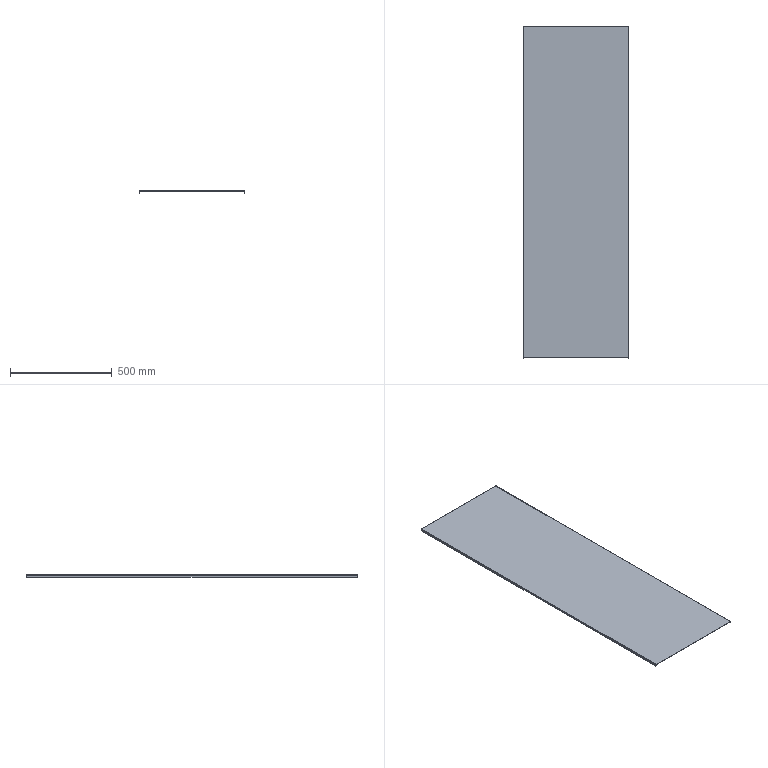Part | STEP file | HESS-408-70-15W-D-12-electrical mounting plate | 1 solid | 18 faces | box 520 x 1630 x 10 mm | volume 1311169 mm3 | plane 10 | cylinder 8 | commonest cylinder face diameters 6 x4 0.2 x2 3.2 x2
STEP:
#1=CARTESIAN_POINT('',(0.,0.,0.));
#2=DIRECTION('',(0.,0.,1.));
#3=DIRECTION('',(1.,0.,0.));
#4=AXIS2_PLACEMENT_3D('',#1,#2,#3);
#5=CARTESIAN_POINT('',(258.4,-815.,-1.5));
#6=VERTEX_POINT('',#5);
#7=CARTESIAN_POINT('',(-258.4,-815.,-1.5));
#8=VERTEX_POINT('',#7);
#9=CARTESIAN_POINT('',(0.,-815.,-1.5));
#10=DIRECTION('',(-1.,0.,0.));
#11=VECTOR('',#10,1.);
#12=LINE('',#9,#11);
#13=CARTESIAN_POINT('',(0.,0.,-1.5));
#14=DIRECTION('',(0.,0.,-1.));
#15=DIRECTION('',(0.,1.,0.));
#16=AXIS2_PLACEMENT_3D('',#13,#14,#15);
#17=PLANE('',#16);
#18=CARTESIAN_POINT('',(-815.,0.));
#19=DIRECTION('',(0.,-1.));
#20=VECTOR('',#19,1.);
#21=LINE('',#18,#20);
#22=(GEOMETRIC_REPRESENTATION_CONTEXT(2)PARAMETRIC_REPRESENTATION_CONTEXT()REPRESENTATION_CONTEXT('',''));
#23=DEFINITIONAL_REPRESENTATION('',(#21),#22);
#24=PCURVE('',#17,#23);
#25=CARTESIAN_POINT('',(-260.,-815.,-1.5));
#26=DIRECTION('',(0.,-1.,0.));
#27=DIRECTION('',(0.,0.,-1.));
#28=AXIS2_PLACEMENT_3D('',#25,#26,#27);
#29=PLANE('',#28);
#30=CARTESIAN_POINT('',(0.,260.));
#31=DIRECTION('',(0.,-1.));
#32=VECTOR('',#31,1.);
#33=LINE('',#30,#32);
#34=(GEOMETRIC_REPRESENTATION_CONTEXT(2)PARAMETRIC_REPRESENTATION_CONTEXT()REPRESENTATION_CONTEXT('',''));
#35=DEFINITIONAL_REPRESENTATION('',(#33),#34);
#36=PCURVE('',#29,#35);
#37=SURFACE_CURVE('',#12,(#24,#36),.PCURVE_S1.);
#38=EDGE_CURVE('',#6,#8,#37,.T.);
#39=ORIENTED_EDGE('',*,*,#38,.T.);
#40=CARTESIAN_POINT('',(-258.4,815.,-1.5));
#41=VERTEX_POINT('',#40);
#42=CARTESIAN_POINT('',(-258.4,0.,-1.5));
#43=DIRECTION('',(0.,1.,0.));
#44=VECTOR('',#43,1.);
#45=LINE('',#42,#44);
#46=CARTESIAN_POINT('',(0.,-258.4));
#47=DIRECTION('',(1.,0.));
#48=VECTOR('',#47,1.);
#49=LINE('',#46,#48);
#50=(GEOMETRIC_REPRESENTATION_CONTEXT(2)PARAMETRIC_REPRESENTATION_CONTEXT()REPRESENTATION_CONTEXT('',''));
#51=DEFINITIONAL_REPRESENTATION('',(#49),#50);
#52=PCURVE('',#17,#51);
#53=CARTESIAN_POINT('',(-258.4,815.,-1.6));
#54=DIRECTION('',(0.,1.,0.));
#55=DIRECTION('',(0.,0.,1.));
#56=AXIS2_PLACEMENT_3D('',#53,#54,#55);
#57=CYLINDRICAL_SURFACE('',#56,0.1);
#58=CARTESIAN_POINT('',(6.283,-815.));
#59=DIRECTION('',(0.,1.));
#60=VECTOR('',#59,1.);
#61=LINE('',#58,#60);
#62=(GEOMETRIC_REPRESENTATION_CONTEXT(2)PARAMETRIC_REPRESENTATION_CONTEXT()REPRESENTATION_CONTEXT('',''));
#63=DEFINITIONAL_REPRESENTATION('',(#61),#62);
#64=PCURVE('',#57,#63);
#65=SURFACE_CURVE('',#45,(#52,#64),.PCURVE_S1.);
#66=EDGE_CURVE('',#8,#41,#65,.T.);
#67=ORIENTED_EDGE('',*,*,#66,.T.);
#68=CARTESIAN_POINT('',(258.4,815.,-1.5));
#69=VERTEX_POINT('',#68);
#70=CARTESIAN_POINT('',(0.,815.,-1.5));
#71=DIRECTION('',(1.,0.,0.));
#72=VECTOR('',#71,1.);
#73=LINE('',#70,#72);
#74=CARTESIAN_POINT('',(815.,0.));
#75=DIRECTION('',(0.,1.));
#76=VECTOR('',#75,1.);
#77=LINE('',#74,#76);
#78=(GEOMETRIC_REPRESENTATION_CONTEXT(2)PARAMETRIC_REPRESENTATION_CONTEXT()REPRESENTATION_CONTEXT('',''));
#79=DEFINITIONAL_REPRESENTATION('',(#77),#78);
#80=PCURVE('',#17,#79);
#81=CARTESIAN_POINT('',(-260.,815.,-1.5));
#82=DIRECTION('',(0.,1.,0.));
#83=DIRECTION('',(0.,0.,1.));
#84=AXIS2_PLACEMENT_3D('',#81,#82,#83);
#85=PLANE('',#84);
#86=CARTESIAN_POINT('',(0.,260.));
#87=DIRECTION('',(0.,1.));
#88=VECTOR('',#87,1.);
#89=LINE('',#86,#88);
#90=(GEOMETRIC_REPRESENTATION_CONTEXT(2)PARAMETRIC_REPRESENTATION_CONTEXT()REPRESENTATION_CONTEXT('',''));
#91=DEFINITIONAL_REPRESENTATION('',(#89),#90);
#92=PCURVE('',#85,#91);
#93=SURFACE_CURVE('',#73,(#80,#92),.PCURVE_S1.);
#94=EDGE_CURVE('',#41,#69,#93,.T.);
#95=ORIENTED_EDGE('',*,*,#94,.T.);
#96=CARTESIAN_POINT('',(258.4,0.,-1.5));
#97=DIRECTION('',(0.,-1.,0.));
#98=VECTOR('',#97,1.);
#99=LINE('',#96,#98);
#100=CARTESIAN_POINT('',(0.,258.4));
#101=DIRECTION('',(-1.,0.));
#102=VECTOR('',#101,1.);
#103=LINE('',#100,#102);
#104=(GEOMETRIC_REPRESENTATION_CONTEXT(2)PARAMETRIC_REPRESENTATION_CONTEXT()REPRESENTATION_CONTEXT('',''));
#105=DEFINITIONAL_REPRESENTATION('',(#103),#104);
#106=PCURVE('',#17,#105);
#107=CARTESIAN_POINT('',(258.4,-815.,-1.6));
#108=DIRECTION('',(0.,-1.,0.));
#109=DIRECTION('',(0.,0.,-1.));
#110=AXIS2_PLACEMENT_3D('',#107,#108,#109);
#111=CYLINDRICAL_SURFACE('',#110,0.1);
#112=CARTESIAN_POINT('',(3.142,-815.));
#113=DIRECTION('',(0.,1.));
#114=VECTOR('',#113,1.);
#115=LINE('',#112,#114);
#116=(GEOMETRIC_REPRESENTATION_CONTEXT(2)PARAMETRIC_REPRESENTATION_CONTEXT()REPRESENTATION_CONTEXT('',''));
#117=DEFINITIONAL_REPRESENTATION('',(#115),#116);
#118=PCURVE('',#111,#117);
#119=SURFACE_CURVE('',#99,(#106,#118),.PCURVE_S1.);
#120=EDGE_CURVE('',#69,#6,#119,.T.);
#121=ORIENTED_EDGE('',*,*,#120,.T.);
#122=EDGE_LOOP('',(#39,#67,#95,#121));
#123=FACE_BOUND('',#122,.T.);
#124=ADVANCED_FACE('',(#123),#17,.T.);
#125=ORIENTED_EDGE('',*,*,#66,.T.);
#126=CARTESIAN_POINT('',(-258.5,815.,-1.6));
#127=VERTEX_POINT('',#126);
#128=CARTESIAN_POINT('',(-258.4,815.,-1.6));
#129=DIRECTION('',(0.,1.,0.));
#130=DIRECTION('',(0.,0.,1.));
#131=AXIS2_PLACEMENT_3D('',#128,#129,#130);
#132=CIRCLE('',#131,0.1);
#133=CARTESIAN_POINT('',(0.,0.));
#134=DIRECTION('',(1.,0.));
#135=VECTOR('',#134,1.);
#136=LINE('',#133,#135);
#137=(GEOMETRIC_REPRESENTATION_CONTEXT(2)PARAMETRIC_REPRESENTATION_CONTEXT()REPRESENTATION_CONTEXT('',''));
#138=DEFINITIONAL_REPRESENTATION('',(#136),#137);
#139=PCURVE('',#57,#138);
#140=CARTESIAN_POINT('',(-0.1,1.6));
#141=DIRECTION('',(1.,0.));
#142=AXIS2_PLACEMENT_2D('',#140,#141);
#143=CIRCLE('',#142,0.1);
#144=(GEOMETRIC_REPRESENTATION_CONTEXT(2)PARAMETRIC_REPRESENTATION_CONTEXT()REPRESENTATION_CONTEXT('',''));
#145=DEFINITIONAL_REPRESENTATION('',(#143),#144);
#146=PCURVE('',#85,#145);
#147=SURFACE_CURVE('',#132,(#139,#146),.PCURVE_S1.);
#148=EDGE_CURVE('',#127,#41,#147,.T.);
#149=ORIENTED_EDGE('',*,*,#148,.F.);
#150=CARTESIAN_POINT('',(-258.5,-815.,-1.6));
#151=VERTEX_POINT('',#150);
#152=CARTESIAN_POINT('',(-258.5,815.,-1.6));
#153=DIRECTION('',(0.,-1.,0.));
#154=VECTOR('',#153,1.);
#155=LINE('',#152,#154);
#156=CARTESIAN_POINT('',(4.712,0.));
#157=DIRECTION('',(0.,-1.));
#158=VECTOR('',#157,1.);
#159=LINE('',#156,#158);
#160=(GEOMETRIC_REPRESENTATION_CONTEXT(2)PARAMETRIC_REPRESENTATION_CONTEXT()REPRESENTATION_CONTEXT('',''));
#161=DEFINITIONAL_REPRESENTATION('',(#159),#160);
#162=PCURVE('',#57,#161);
#163=CARTESIAN_POINT('',(-258.5,0.,0.));
#164=DIRECTION('',(-1.,0.,0.));
#165=DIRECTION('',(0.,0.,1.));
#166=AXIS2_PLACEMENT_3D('',#163,#164,#165);
#167=PLANE('',#166);
#168=CARTESIAN_POINT('',(-1.6,815.));
#169=DIRECTION('',(0.,-1.));
#170=VECTOR('',#169,1.);
#171=LINE('',#168,#170);
#172=(GEOMETRIC_REPRESENTATION_CONTEXT(2)PARAMETRIC_REPRESENTATION_CONTEXT()REPRESENTATION_CONTEXT('',''));
#173=DEFINITIONAL_REPRESENTATION('',(#171),#172);
#174=PCURVE('',#167,#173);
#175=SURFACE_CURVE('',#155,(#162,#174),.PCURVE_S1.);
#176=EDGE_CURVE('',#127,#151,#175,.T.);
#177=ORIENTED_EDGE('',*,*,#176,.T.);
#178=CARTESIAN_POINT('',(-258.4,-815.,-1.6));
#179=DIRECTION('',(0.,1.,0.));
#180=DIRECTION('',(0.,0.,1.));
#181=AXIS2_PLACEMENT_3D('',#178,#179,#180);
#182=CIRCLE('',#181,0.1);
#183=CARTESIAN_POINT('',(0.,-1630.));
#184=DIRECTION('',(1.,0.));
#185=VECTOR('',#184,1.);
#186=LINE('',#183,#185);
#187=(GEOMETRIC_REPRESENTATION_CONTEXT(2)PARAMETRIC_REPRESENTATION_CONTEXT()REPRESENTATION_CONTEXT('',''));
#188=DEFINITIONAL_REPRESENTATION('',(#186),#187);
#189=PCURVE('',#57,#188);
#190=CARTESIAN_POINT('',(0.,1.6));
#191=CARTESIAN_POINT('',(0.,1.773));
#192=CARTESIAN_POINT('',(0.15,1.687));
#193=CARTESIAN_POINT('',(0.3,1.6));
#194=CARTESIAN_POINT('',(0.15,1.513));
#195=CARTESIAN_POINT('',(0.,1.427));
#196=CARTESIAN_POINT('',(0.,1.6));
#197=(BOUNDED_CURVE()B_SPLINE_CURVE(2,(#190,#191,#192,#193,#194,#195,#196),.UNSPECIFIED.,.T.,.F.)B_SPLINE_CURVE_WITH_KNOTS((1,2,2,2,2,1),(-2.094,0.,2.094,4.189,6.283,8.378),.UNSPECIFIED.)CURVE()GEOMETRIC_REPRESENTATION_ITEM()RATIONAL_B_SPLINE_CURVE((1.,0.5,1.,0.5,1.,0.5,1.))REPRESENTATION_ITEM(''));
#198=(GEOMETRIC_REPRESENTATION_CONTEXT(2)PARAMETRIC_REPRESENTATION_CONTEXT()REPRESENTATION_CONTEXT('',''));
#199=DEFINITIONAL_REPRESENTATION('',(#197),#198);
#200=PCURVE('',#29,#199);
#201=SURFACE_CURVE('',#182,(#189,#200),.PCURVE_S1.);
#202=EDGE_CURVE('',#151,#8,#201,.T.);
#203=ORIENTED_EDGE('',*,*,#202,.T.);
#204=EDGE_LOOP('',(#125,#149,#177,#203));
#205=FACE_BOUND('',#204,.F.);
#206=ADVANCED_FACE('',(#205),#57,.F.);
#207=CARTESIAN_POINT('',(258.4,-815.,0.));
#208=VERTEX_POINT('',#207);
#209=CARTESIAN_POINT('',(-258.4,-815.,0.));
#210=VERTEX_POINT('',#209);
#211=CARTESIAN_POINT('',(-260.,-815.,0.));
#212=DIRECTION('',(-1.,0.,0.));
#213=VECTOR('',#212,1.);
#214=LINE('',#211,#213);
#215=CARTESIAN_POINT('',(-1.5,0.));
#216=DIRECTION('',(0.,-1.));
#217=VECTOR('',#216,1.);
#218=LINE('',#215,#217);
#219=(GEOMETRIC_REPRESENTATION_CONTEXT(2)PARAMETRIC_REPRESENTATION_CONTEXT()REPRESENTATION_CONTEXT('',''));
#220=DEFINITIONAL_REPRESENTATION('',(#218),#219);
#221=PCURVE('',#29,#220);
#222=CARTESIAN_POINT('',(0.,0.,0.));
#223=DIRECTION('',(0.,0.,-1.));
#224=DIRECTION('',(0.,1.,0.));
#225=AXIS2_PLACEMENT_3D('',#222,#223,#224);
#226=PLANE('',#225);
#227=CARTESIAN_POINT('',(-815.,-260.));
#228=DIRECTION('',(0.,-1.));
#229=VECTOR('',#228,1.);
#230=LINE('',#227,#229);
#231=(GEOMETRIC_REPRESENTATION_CONTEXT(2)PARAMETRIC_REPRESENTATION_CONTEXT()REPRESENTATION_CONTEXT('',''));
#232=DEFINITIONAL_REPRESENTATION('',(#230),#231);
#233=PCURVE('',#226,#232);
#234=SURFACE_CURVE('',#214,(#221,#233),.PCURVE_S1.);
#235=EDGE_CURVE('',#208,#210,#234,.T.);
#236=ORIENTED_EDGE('',*,*,#235,.T.);
#237=CARTESIAN_POINT('',(-260.,-815.,-1.6));
#238=VERTEX_POINT('',#237);
#239=CARTESIAN_POINT('',(-258.4,-815.,-1.6));
#240=DIRECTION('',(0.,1.,0.));
#241=DIRECTION('',(0.,0.,1.));
#242=AXIS2_PLACEMENT_3D('',#239,#240,#241);
#243=CIRCLE('',#242,1.6);
#244=CARTESIAN_POINT('',(-1.5,1.6));
#245=CARTESIAN_POINT('',(-1.5,4.371));
#246=CARTESIAN_POINT('',(0.9,2.986));
#247=CARTESIAN_POINT('',(3.3,1.6));
#248=CARTESIAN_POINT('',(0.9,0.2144));
#249=CARTESIAN_POINT('',(-1.5,-1.171));
#250=CARTESIAN_POINT('',(-1.5,1.6));
#251=(BOUNDED_CURVE()B_SPLINE_CURVE(2,(#244,#245,#246,#247,#248,#249,#250),.UNSPECIFIED.,.T.,.F.)B_SPLINE_CURVE_WITH_KNOTS((1,2,2,2,2,1),(-2.094,0.,2.094,4.189,6.283,8.378),.UNSPECIFIED.)CURVE()GEOMETRIC_REPRESENTATION_ITEM()RATIONAL_B_SPLINE_CURVE((1.,0.5,1.,0.5,1.,0.5,1.))REPRESENTATION_ITEM(''));
#252=(GEOMETRIC_REPRESENTATION_CONTEXT(2)PARAMETRIC_REPRESENTATION_CONTEXT()REPRESENTATION_CONTEXT('',''));
#253=DEFINITIONAL_REPRESENTATION('',(#251),#252);
#254=PCURVE('',#29,#253);
#255=CARTESIAN_POINT('',(-258.4,815.,-1.6));
#256=DIRECTION('',(0.,1.,0.));
#257=DIRECTION('',(0.,0.,1.));
#258=AXIS2_PLACEMENT_3D('',#255,#256,#257);
#259=CYLINDRICAL_SURFACE('',#258,1.6);
#260=CARTESIAN_POINT('',(0.,-1630.));
#261=DIRECTION('',(1.,0.));
#262=VECTOR('',#261,1.);
#263=LINE('',#260,#262);
#264=(GEOMETRIC_REPRESENTATION_CONTEXT(2)PARAMETRIC_REPRESENTATION_CONTEXT()REPRESENTATION_CONTEXT('',''));
#265=DEFINITIONAL_REPRESENTATION('',(#263),#264);
#266=PCURVE('',#259,#265);
#267=SURFACE_CURVE('',#243,(#254,#266),.PCURVE_S1.);
#268=EDGE_CURVE('',#238,#210,#267,.T.);
#269=ORIENTED_EDGE('',*,*,#268,.F.);
#270=CARTESIAN_POINT('',(-260.,-815.,-7.));
#271=VERTEX_POINT('',#270);
#272=CARTESIAN_POINT('',(-260.,-815.,-10.));
#273=DIRECTION('',(0.,0.,-1.));
#274=VECTOR('',#273,1.);
#275=LINE('',#272,#274);
#276=CARTESIAN_POINT('',(8.5,0.));
#277=DIRECTION('',(1.,0.));
#278=VECTOR('',#277,1.);
#279=LINE('',#276,#278);
#280=(GEOMETRIC_REPRESENTATION_CONTEXT(2)PARAMETRIC_REPRESENTATION_CONTEXT()REPRESENTATION_CONTEXT('',''));
#281=DEFINITIONAL_REPRESENTATION('',(#279),#280);
#282=PCURVE('',#29,#281);
#283=CARTESIAN_POINT('',(-260.,0.,0.));
#284=DIRECTION('',(-1.,0.,0.));
#285=DIRECTION('',(0.,0.,1.));
#286=AXIS2_PLACEMENT_3D('',#283,#284,#285);
#287=PLANE('',#286);
#288=CARTESIAN_POINT('',(-10.,-815.));
#289=DIRECTION('',(-1.,0.));
#290=VECTOR('',#289,1.);
#291=LINE('',#288,#290);
#292=(GEOMETRIC_REPRESENTATION_CONTEXT(2)PARAMETRIC_REPRESENTATION_CONTEXT()REPRESENTATION_CONTEXT('',''));
#293=DEFINITIONAL_REPRESENTATION('',(#291),#292);
#294=PCURVE('',#287,#293);
#295=SURFACE_CURVE('',#275,(#282,#294),.PCURVE_S1.);
#296=EDGE_CURVE('',#238,#271,#295,.T.);
#297=ORIENTED_EDGE('',*,*,#296,.T.);
#298=CARTESIAN_POINT('',(-258.5,-815.,-7.));
#299=VERTEX_POINT('',#298);
#300=CARTESIAN_POINT('',(-260.,-815.,-7.));
#301=DIRECTION('',(1.,0.,0.));
#302=VECTOR('',#301,1.);
#303=LINE('',#300,#302);
#304=CARTESIAN_POINT('',(5.5,0.));
#305=DIRECTION('',(0.,1.));
#306=VECTOR('',#305,1.);
#307=LINE('',#304,#306);
#308=(GEOMETRIC_REPRESENTATION_CONTEXT(2)PARAMETRIC_REPRESENTATION_CONTEXT()REPRESENTATION_CONTEXT('',''));
#309=DEFINITIONAL_REPRESENTATION('',(#307),#308);
#310=PCURVE('',#29,#309);
#311=CARTESIAN_POINT('',(-260.,-812.,-7.));
#312=DIRECTION('',(1.,0.,0.));
#313=DIRECTION('',(0.,0.,-1.));
#314=AXIS2_PLACEMENT_3D('',#311,#312,#313);
#315=CYLINDRICAL_SURFACE('',#314,3.);
#316=CARTESIAN_POINT('',(4.712,0.));
#317=DIRECTION('',(0.,1.));
#318=VECTOR('',#317,1.);
#319=LINE('',#316,#318);
#320=(GEOMETRIC_REPRESENTATION_CONTEXT(2)PARAMETRIC_REPRESENTATION_CONTEXT()REPRESENTATION_CONTEXT('',''));
#321=DEFINITIONAL_REPRESENTATION('',(#319),#320);
#322=PCURVE('',#315,#321);
#323=SURFACE_CURVE('',#303,(#310,#322),.PCURVE_S1.);
#324=EDGE_CURVE('',#271,#299,#323,.T.);
#325=ORIENTED_EDGE('',*,*,#324,.T.);
#326=CARTESIAN_POINT('',(-258.5,-815.,0.));
#327=DIRECTION('',(0.,0.,1.));
#328=VECTOR('',#327,1.);
#329=LINE('',#326,#328);
#330=CARTESIAN_POINT('',(-1.5,1.5));
#331=DIRECTION('',(-1.,0.));
#332=VECTOR('',#331,1.);
#333=LINE('',#330,#332);
#334=(GEOMETRIC_REPRESENTATION_CONTEXT(2)PARAMETRIC_REPRESENTATION_CONTEXT()REPRESENTATION_CONTEXT('',''));
#335=DEFINITIONAL_REPRESENTATION('',(#333),#334);
#336=PCURVE('',#29,#335);
#337=CARTESIAN_POINT('',(0.,-815.));
#338=DIRECTION('',(1.,0.));
#339=VECTOR('',#338,1.);
#340=LINE('',#337,#339);
#341=(GEOMETRIC_REPRESENTATION_CONTEXT(2)PARAMETRIC_REPRESENTATION_CONTEXT()REPRESENTATION_CONTEXT('',''));
#342=DEFINITIONAL_REPRESENTATION('',(#340),#341);
#343=PCURVE('',#167,#342);
#344=SURFACE_CURVE('',#329,(#336,#343),.PCURVE_S1.);
#345=EDGE_CURVE('',#299,#151,#344,.T.);
#346=ORIENTED_EDGE('',*,*,#345,.T.);
#347=ORIENTED_EDGE('',*,*,#202,.T.);
#348=ORIENTED_EDGE('',*,*,#38,.F.);
#349=CARTESIAN_POINT('',(258.5,-815.,-1.6));
#350=VERTEX_POINT('',#349);
#351=CARTESIAN_POINT('',(258.4,-815.,-1.6));
#352=DIRECTION('',(0.,-1.,0.));
#353=DIRECTION('',(0.,0.,-1.));
#354=AXIS2_PLACEMENT_3D('',#351,#352,#353);
#355=CIRCLE('',#354,0.1);
#356=CARTESIAN_POINT('',(0.1,518.4));
#357=DIRECTION('',(1.,0.));
#358=AXIS2_PLACEMENT_2D('',#356,#357);
#359=CIRCLE('',#358,0.1);
#360=(GEOMETRIC_REPRESENTATION_CONTEXT(2)PARAMETRIC_REPRESENTATION_CONTEXT()REPRESENTATION_CONTEXT('',''));
#361=DEFINITIONAL_REPRESENTATION('',(#359),#360);
#362=PCURVE('',#29,#361);
#363=CARTESIAN_POINT('',(0.,0.));
#364=DIRECTION('',(1.,0.));
#365=VECTOR('',#364,1.);
#366=LINE('',#363,#365);
#367=(GEOMETRIC_REPRESENTATION_CONTEXT(2)PARAMETRIC_REPRESENTATION_CONTEXT()REPRESENTATION_CONTEXT('',''));
#368=DEFINITIONAL_REPRESENTATION('',(#366),#367);
#369=PCURVE('',#111,#368);
#370=SURFACE_CURVE('',#355,(#362,#369),.PCURVE_S1.);
#371=EDGE_CURVE('',#350,#6,#370,.T.);
#372=ORIENTED_EDGE('',*,*,#371,.F.);
#373=CARTESIAN_POINT('',(258.5,-815.,-7.));
#374=VERTEX_POINT('',#373);
#375=CARTESIAN_POINT('',(258.5,-815.,0.));
#376=DIRECTION('',(0.,0.,1.));
#377=VECTOR('',#376,1.);
#378=LINE('',#375,#377);
#379=CARTESIAN_POINT('',(-1.5,518.5));
#380=DIRECTION('',(-1.,0.));
#381=VECTOR('',#380,1.);
#382=LINE('',#379,#381);
#383=(GEOMETRIC_REPRESENTATION_CONTEXT(2)PARAMETRIC_REPRESENTATION_CONTEXT()REPRESENTATION_CONTEXT('',''));
#384=DEFINITIONAL_REPRESENTATION('',(#382),#383);
#385=PCURVE('',#29,#384);
#386=CARTESIAN_POINT('',(258.5,0.,0.));
#387=DIRECTION('',(-1.,0.,0.));
#388=DIRECTION('',(0.,0.,1.));
#389=AXIS2_PLACEMENT_3D('',#386,#387,#388);
#390=PLANE('',#389);
#391=CARTESIAN_POINT('',(0.,-815.));
#392=DIRECTION('',(1.,0.));
#393=VECTOR('',#392,1.);
#394=LINE('',#391,#393);
#395=(GEOMETRIC_REPRESENTATION_CONTEXT(2)PARAMETRIC_REPRESENTATION_CONTEXT()REPRESENTATION_CONTEXT('',''));
#396=DEFINITIONAL_REPRESENTATION('',(#394),#395);
#397=PCURVE('',#390,#396);
#398=SURFACE_CURVE('',#378,(#385,#397),.PCURVE_S1.);
#399=EDGE_CURVE('',#374,#350,#398,.T.);
#400=ORIENTED_EDGE('',*,*,#399,.F.);
#401=CARTESIAN_POINT('',(260.,-815.,-7.));
#402=VERTEX_POINT('',#401);
#403=CARTESIAN_POINT('',(260.,-815.,-7.));
#404=DIRECTION('',(1.,0.,0.));
#405=VECTOR('',#404,1.);
#406=LINE('',#403,#405);
#407=CARTESIAN_POINT('',(5.5,520.));
#408=DIRECTION('',(0.,1.));
#409=VECTOR('',#408,1.);
#410=LINE('',#407,#409);
#411=(GEOMETRIC_REPRESENTATION_CONTEXT(2)PARAMETRIC_REPRESENTATION_CONTEXT()REPRESENTATION_CONTEXT('',''));
#412=DEFINITIONAL_REPRESENTATION('',(#410),#411);
#413=PCURVE('',#29,#412);
#414=CARTESIAN_POINT('',(260.,-812.,-7.));
#415=DIRECTION('',(-1.,0.,0.));
#416=DIRECTION('',(0.,0.,1.));
#417=AXIS2_PLACEMENT_3D('',#414,#415,#416);
#418=CYLINDRICAL_SURFACE('',#417,3.);
#419=CARTESIAN_POINT('',(4.712,0.));
#420=DIRECTION('',(0.,-1.));
#421=VECTOR('',#420,1.);
#422=LINE('',#419,#421);
#423=(GEOMETRIC_REPRESENTATION_CONTEXT(2)PARAMETRIC_REPRESENTATION_CONTEXT()REPRESENTATION_CONTEXT('',''));
#424=DEFINITIONAL_REPRESENTATION('',(#422),#423);
#425=PCURVE('',#418,#424);
#426=SURFACE_CURVE('',#406,(#413,#425),.PCURVE_S1.);
#427=EDGE_CURVE('',#374,#402,#426,.T.);
#428=ORIENTED_EDGE('',*,*,#427,.T.);
#429=CARTESIAN_POINT('',(260.,-815.,-1.6));
#430=VERTEX_POINT('',#429);
#431=CARTESIAN_POINT('',(260.,-815.,-10.));
#432=DIRECTION('',(0.,0.,1.));
#433=VECTOR('',#432,1.);
#434=LINE('',#431,#433);
#435=CARTESIAN_POINT('',(8.5,520.));
#436=DIRECTION('',(-1.,0.));
#437=VECTOR('',#436,1.);
#438=LINE('',#435,#437);
#439=(GEOMETRIC_REPRESENTATION_CONTEXT(2)PARAMETRIC_REPRESENTATION_CONTEXT()REPRESENTATION_CONTEXT('',''));
#440=DEFINITIONAL_REPRESENTATION('',(#438),#439);
#441=PCURVE('',#29,#440);
#442=CARTESIAN_POINT('',(260.,0.,0.));
#443=DIRECTION('',(-1.,0.,0.));
#444=DIRECTION('',(0.,0.,1.));
#445=AXIS2_PLACEMENT_3D('',#442,#443,#444);
#446=PLANE('',#445);
#447=CARTESIAN_POINT('',(-10.,-815.));
#448=DIRECTION('',(1.,0.));
#449=VECTOR('',#448,1.);
#450=LINE('',#447,#449);
#451=(GEOMETRIC_REPRESENTATION_CONTEXT(2)PARAMETRIC_REPRESENTATION_CONTEXT()REPRESENTATION_CONTEXT('',''));
#452=DEFINITIONAL_REPRESENTATION('',(#450),#451);
#453=PCURVE('',#446,#452);
#454=SURFACE_CURVE('',#434,(#441,#453),.PCURVE_S1.);
#455=EDGE_CURVE('',#402,#430,#454,.T.);
#456=ORIENTED_EDGE('',*,*,#455,.T.);
#457=CARTESIAN_POINT('',(258.4,-815.,-1.6));
#458=DIRECTION('',(0.,1.,0.));
#459=DIRECTION('',(0.,0.,-1.));
#460=AXIS2_PLACEMENT_3D('',#457,#458,#459);
#461=CIRCLE('',#460,1.6);
#462=CARTESIAN_POINT('',(1.7,518.4));
#463=CARTESIAN_POINT('',(1.7,515.629));
#464=CARTESIAN_POINT('',(-0.7,517.014));
#465=CARTESIAN_POINT('',(-3.1,518.4));
#466=CARTESIAN_POINT('',(-0.7,519.786));
#467=CARTESIAN_POINT('',(1.7,521.171));
#468=CARTESIAN_POINT('',(1.7,518.4));
#469=(BOUNDED_CURVE()B_SPLINE_CURVE(2,(#462,#463,#464,#465,#466,#467,#468),.UNSPECIFIED.,.T.,.F.)B_SPLINE_CURVE_WITH_KNOTS((1,2,2,2,2,1),(-2.094,0.,2.094,4.189,6.283,8.378),.UNSPECIFIED.)CURVE()GEOMETRIC_REPRESENTATION_ITEM()RATIONAL_B_SPLINE_CURVE((1.,0.5,1.,0.5,1.,0.5,1.))REPRESENTATION_ITEM(''));
#470=(GEOMETRIC_REPRESENTATION_CONTEXT(2)PARAMETRIC_REPRESENTATION_CONTEXT()REPRESENTATION_CONTEXT('',''));
#471=DEFINITIONAL_REPRESENTATION('',(#469),#470);
#472=PCURVE('',#29,#471);
#473=CARTESIAN_POINT('',(258.4,-815.,-1.6));
#474=DIRECTION('',(0.,-1.,0.));
#475=DIRECTION('',(0.,0.,-1.));
#476=AXIS2_PLACEMENT_3D('',#473,#474,#475);
#477=CYLINDRICAL_SURFACE('',#476,1.6);
#478=CARTESIAN_POINT('',(6.283,0.));
#479=DIRECTION('',(-1.,0.));
#480=VECTOR('',#479,1.);
#481=LINE('',#478,#480);
#482=(GEOMETRIC_REPRESENTATION_CONTEXT(2)PARAMETRIC_REPRESENTATION_CONTEXT()REPRESENTATION_CONTEXT('',''));
#483=DEFINITIONAL_REPRESENTATION('',(#481),#482);
#484=PCURVE('',#477,#483);
#485=SURFACE_CURVE('',#461,(#472,#484),.PCURVE_S1.);
#486=EDGE_CURVE('',#208,#430,#485,.T.);
#487=ORIENTED_EDGE('',*,*,#486,.F.);
#488=EDGE_LOOP('',(#236,#269,#297,#325,#346,#347,#348,#372,#400,#428,#456,#487));
#489=FACE_BOUND('',#488,.T.);
#490=ADVANCED_FACE('',(#489),#29,.T.);
#491=ORIENTED_EDGE('',*,*,#120,.T.);
#492=ORIENTED_EDGE('',*,*,#371,.F.);
#493=CARTESIAN_POINT('',(258.5,815.,-1.6));
#494=VERTEX_POINT('',#493);
#495=CARTESIAN_POINT('',(258.5,-815.,-1.6));
#496=DIRECTION('',(0.,1.,0.));
#497=VECTOR('',#496,1.);
#498=LINE('',#495,#497);
#499=CARTESIAN_POINT('',(1.571,0.));
#500=DIRECTION('',(0.,-1.));
#501=VECTOR('',#500,1.);
#502=LINE('',#499,#501);
#503=(GEOMETRIC_REPRESENTATION_CONTEXT(2)PARAMETRIC_REPRESENTATION_CONTEXT()REPRESENTATION_CONTEXT('',''));
#504=DEFINITIONAL_REPRESENTATION('',(#502),#503);
#505=PCURVE('',#111,#504);
#506=CARTESIAN_POINT('',(-1.6,-815.));
#507=DIRECTION('',(0.,1.));
#508=VECTOR('',#507,1.);
#509=LINE('',#506,#508);
#510=(GEOMETRIC_REPRESENTATION_CONTEXT(2)PARAMETRIC_REPRESENTATION_CONTEXT()REPRESENTATION_CONTEXT('',''));
#511=DEFINITIONAL_REPRESENTATION('',(#509),#510);
#512=PCURVE('',#390,#511);
#513=SURFACE_CURVE('',#498,(#505,#512),.PCURVE_S1.);
#514=EDGE_CURVE('',#350,#494,#513,.T.);
#515=ORIENTED_EDGE('',*,*,#514,.T.);
#516=CARTESIAN_POINT('',(258.4,815.,-1.6));
#517=DIRECTION('',(0.,-1.,0.));
#518=DIRECTION('',(0.,0.,-1.));
#519=AXIS2_PLACEMENT_3D('',#516,#517,#518);
#520=CIRCLE('',#519,0.1);
#521=CARTESIAN_POINT('',(0.,-1630.));
#522=DIRECTION('',(1.,0.));
#523=VECTOR('',#522,1.);
#524=LINE('',#521,#523);
#525=(GEOMETRIC_REPRESENTATION_CONTEXT(2)PARAMETRIC_REPRESENTATION_CONTEXT()REPRESENTATION_CONTEXT('',''));
#526=DEFINITIONAL_REPRESENTATION('',(#524),#525);
#527=PCURVE('',#111,#526);
#528=CARTESIAN_POINT('',(-0.2,518.4));
#529=CARTESIAN_POINT('',(-0.2,518.573));
#530=CARTESIAN_POINT('',(-0.05,518.487));
#531=CARTESIAN_POINT('',(0.1,518.4));
#532=CARTESIAN_POINT('',(-0.05,518.313));
#533=CARTESIAN_POINT('',(-0.2,518.227));
#534=CARTESIAN_POINT('',(-0.2,518.4));
#535=(BOUNDED_CURVE()B_SPLINE_CURVE(2,(#528,#529,#530,#531,#532,#533,#534),.UNSPECIFIED.,.T.,.F.)B_SPLINE_CURVE_WITH_KNOTS((1,2,2,2,2,1),(-2.094,0.,2.094,4.189,6.283,8.378),.UNSPECIFIED.)CURVE()GEOMETRIC_REPRESENTATION_ITEM()RATIONAL_B_SPLINE_CURVE((1.,0.5,1.,0.5,1.,0.5,1.))REPRESENTATION_ITEM(''));
#536=(GEOMETRIC_REPRESENTATION_CONTEXT(2)PARAMETRIC_REPRESENTATION_CONTEXT()REPRESENTATION_CONTEXT('',''));
#537=DEFINITIONAL_REPRESENTATION('',(#535),#536);
#538=PCURVE('',#85,#537);
#539=SURFACE_CURVE('',#520,(#527,#538),.PCURVE_S1.);
#540=EDGE_CURVE('',#494,#69,#539,.T.);
#541=ORIENTED_EDGE('',*,*,#540,.T.);
#542=EDGE_LOOP('',(#491,#492,#515,#541));
#543=FACE_BOUND('',#542,.F.);
#544=ADVANCED_FACE('',(#543),#111,.F.);
#545=ORIENTED_EDGE('',*,*,#94,.F.);
#546=ORIENTED_EDGE('',*,*,#148,.F.);
#547=CARTESIAN_POINT('',(-258.5,815.,-7.));
#548=VERTEX_POINT('',#547);
#549=CARTESIAN_POINT('',(-258.5,815.,0.));
#550=DIRECTION('',(0.,0.,-1.));
#551=VECTOR('',#550,1.);
#552=LINE('',#549,#551);
#553=CARTESIAN_POINT('',(1.5,1.5));
#554=DIRECTION('',(-1.,0.));
#555=VECTOR('',#554,1.);
#556=LINE('',#553,#555);
#557=(GEOMETRIC_REPRESENTATION_CONTEXT(2)PARAMETRIC_REPRESENTATION_CONTEXT()REPRESENTATION_CONTEXT('',''));
#558=DEFINITIONAL_REPRESENTATION('',(#556),#557);
#559=PCURVE('',#85,#558);
#560=CARTESIAN_POINT('',(0.,815.));
#561=DIRECTION('',(-1.,0.));
#562=VECTOR('',#561,1.);
#563=LINE('',#560,#562);
#564=(GEOMETRIC_REPRESENTATION_CONTEXT(2)PARAMETRIC_REPRESENTATION_CONTEXT()REPRESENTATION_CONTEXT('',''));
#565=DEFINITIONAL_REPRESENTATION('',(#563),#564);
#566=PCURVE('',#167,#565);
#567=SURFACE_CURVE('',#552,(#559,#566),.PCURVE_S1.);
#568=EDGE_CURVE('',#127,#548,#567,.T.);
#569=ORIENTED_EDGE('',*,*,#568,.T.);
#570=CARTESIAN_POINT('',(-260.,815.,-7.));
#571=VERTEX_POINT('',#570);
#572=CARTESIAN_POINT('',(-260.,815.,-7.));
#573=DIRECTION('',(1.,0.,0.));
#574=VECTOR('',#573,1.);
#575=LINE('',#572,#574);
#576=CARTESIAN_POINT('',(-5.5,0.));
#577=DIRECTION('',(0.,1.));
#578=VECTOR('',#577,1.);
#579=LINE('',#576,#578);
#580=(GEOMETRIC_REPRESENTATION_CONTEXT(2)PARAMETRIC_REPRESENTATION_CONTEXT()REPRESENTATION_CONTEXT('',''));
#581=DEFINITIONAL_REPRESENTATION('',(#579),#580);
#582=PCURVE('',#85,#581);
#583=CARTESIAN_POINT('',(-260.,812.,-7.));
#584=DIRECTION('',(1.,0.,0.));
#585=DIRECTION('',(0.,0.,-1.));
#586=AXIS2_PLACEMENT_3D('',#583,#584,#585);
#587=CYLINDRICAL_SURFACE('',#586,3.);
#588=CARTESIAN_POINT('',(1.571,0.));
#589=DIRECTION('',(0.,1.));
#590=VECTOR('',#589,1.);
#591=LINE('',#588,#590);
#592=(GEOMETRIC_REPRESENTATION_CONTEXT(2)PARAMETRIC_REPRESENTATION_CONTEXT()REPRESENTATION_CONTEXT('',''));
#593=DEFINITIONAL_REPRESENTATION('',(#591),#592);
#594=PCURVE('',#587,#593);
#595=SURFACE_CURVE('',#575,(#582,#594),.PCURVE_S1.);
#596=EDGE_CURVE('',#571,#548,#595,.T.);
#597=ORIENTED_EDGE('',*,*,#596,.F.);
#598=CARTESIAN_POINT('',(-260.,815.,-1.6));
#599=VERTEX_POINT('',#598);
#600=CARTESIAN_POINT('',(-260.,815.,-1.5));
#601=DIRECTION('',(0.,0.,1.));
#602=VECTOR('',#601,1.);
#603=LINE('',#600,#602);
#604=CARTESIAN_POINT('',(0.,0.));
#605=DIRECTION('',(1.,0.));
#606=VECTOR('',#605,1.);
#607=LINE('',#604,#606);
#608=(GEOMETRIC_REPRESENTATION_CONTEXT(2)PARAMETRIC_REPRESENTATION_CONTEXT()REPRESENTATION_CONTEXT('',''));
#609=DEFINITIONAL_REPRESENTATION('',(#607),#608);
#610=PCURVE('',#85,#609);
#611=CARTESIAN_POINT('',(-1.5,815.));
#612=DIRECTION('',(1.,0.));
#613=VECTOR('',#612,1.);
#614=LINE('',#611,#613);
#615=(GEOMETRIC_REPRESENTATION_CONTEXT(2)PARAMETRIC_REPRESENTATION_CONTEXT()REPRESENTATION_CONTEXT('',''));
#616=DEFINITIONAL_REPRESENTATION('',(#614),#615);
#617=PCURVE('',#287,#616);
#618=SURFACE_CURVE('',#603,(#610,#617),.PCURVE_S1.);
#619=EDGE_CURVE('',#571,#599,#618,.T.);
#620=ORIENTED_EDGE('',*,*,#619,.T.);
#621=CARTESIAN_POINT('',(-258.4,815.,0.));
#622=VERTEX_POINT('',#621);
#623=CARTESIAN_POINT('',(-258.4,815.,-1.6));
#624=DIRECTION('',(0.,-1.,0.));
#625=DIRECTION('',(0.,0.,1.));
#626=AXIS2_PLACEMENT_3D('',#623,#624,#625);
#627=CIRCLE('',#626,1.6);
#628=CARTESIAN_POINT('',(1.5,1.6));
#629=CARTESIAN_POINT('',(1.5,-1.171));
#630=CARTESIAN_POINT('',(-0.9,0.2144));
#631=CARTESIAN_POINT('',(-3.3,1.6));
#632=CARTESIAN_POINT('',(-0.9,2.986));
#633=CARTESIAN_POINT('',(1.5,4.371));
#634=CARTESIAN_POINT('',(1.5,1.6));
#635=(BOUNDED_CURVE()B_SPLINE_CURVE(2,(#628,#629,#630,#631,#632,#633,#634),.UNSPECIFIED.,.T.,.F.)B_SPLINE_CURVE_WITH_KNOTS((1,2,2,2,2,1),(-2.094,0.,2.094,4.189,6.283,8.378),.UNSPECIFIED.)CURVE()GEOMETRIC_REPRESENTATION_ITEM()RATIONAL_B_SPLINE_CURVE((1.,0.5,1.,0.5,1.,0.5,1.))REPRESENTATION_ITEM(''));
#636=(GEOMETRIC_REPRESENTATION_CONTEXT(2)PARAMETRIC_REPRESENTATION_CONTEXT()REPRESENTATION_CONTEXT('',''));
#637=DEFINITIONAL_REPRESENTATION('',(#635),#636);
#638=PCURVE('',#85,#637);
#639=CARTESIAN_POINT('',(6.283,0.));
#640=DIRECTION('',(-1.,0.));
#641=VECTOR('',#640,1.);
#642=LINE('',#639,#641);
#643=(GEOMETRIC_REPRESENTATION_CONTEXT(2)PARAMETRIC_REPRESENTATION_CONTEXT()REPRESENTATION_CONTEXT('',''));
#644=DEFINITIONAL_REPRESENTATION('',(#642),#643);
#645=PCURVE('',#259,#644);
#646=SURFACE_CURVE('',#627,(#638,#645),.PCURVE_S1.);
#647=EDGE_CURVE('',#622,#599,#646,.T.);
#648=ORIENTED_EDGE('',*,*,#647,.F.);
#649=CARTESIAN_POINT('',(258.4,815.,0.));
#650=VERTEX_POINT('',#649);
#651=CARTESIAN_POINT('',(-260.,815.,0.));
#652=DIRECTION('',(1.,0.,0.));
#653=VECTOR('',#652,1.);
#654=LINE('',#651,#653);
#655=CARTESIAN_POINT('',(1.5,0.));
#656=DIRECTION('',(0.,1.));
#657=VECTOR('',#656,1.);
#658=LINE('',#655,#657);
#659=(GEOMETRIC_REPRESENTATION_CONTEXT(2)PARAMETRIC_REPRESENTATION_CONTEXT()REPRESENTATION_CONTEXT('',''));
#660=DEFINITIONAL_REPRESENTATION('',(#658),#659);
#661=PCURVE('',#85,#660);
#662=CARTESIAN_POINT('',(815.,-260.));
#663=DIRECTION('',(0.,1.));
#664=VECTOR('',#663,1.);
#665=LINE('',#662,#664);
#666=(GEOMETRIC_REPRESENTATION_CONTEXT(2)PARAMETRIC_REPRESENTATION_CONTEXT()REPRESENTATION_CONTEXT('',''));
#667=DEFINITIONAL_REPRESENTATION('',(#665),#666);
#668=PCURVE('',#226,#667);
#669=SURFACE_CURVE('',#654,(#661,#668),.PCURVE_S1.);
#670=EDGE_CURVE('',#622,#650,#669,.T.);
#671=ORIENTED_EDGE('',*,*,#670,.T.);
#672=CARTESIAN_POINT('',(260.,815.,-1.6));
#673=VERTEX_POINT('',#672);
#674=CARTESIAN_POINT('',(258.4,815.,-1.6));
#675=DIRECTION('',(0.,-1.,0.));
#676=DIRECTION('',(0.,0.,-1.));
#677=AXIS2_PLACEMENT_3D('',#674,#675,#676);
#678=CIRCLE('',#677,1.6);
#679=CARTESIAN_POINT('',(-1.7,518.4));
#680=CARTESIAN_POINT('',(-1.7,521.171));
#681=CARTESIAN_POINT('',(0.7,519.786));
#682=CARTESIAN_POINT('',(3.1,518.4));
#683=CARTESIAN_POINT('',(0.7,517.014));
#684=CARTESIAN_POINT('',(-1.7,515.629));
#685=CARTESIAN_POINT('',(-1.7,518.4));
#686=(BOUNDED_CURVE()B_SPLINE_CURVE(2,(#679,#680,#681,#682,#683,#684,#685),.UNSPECIFIED.,.T.,.F.)B_SPLINE_CURVE_WITH_KNOTS((1,2,2,2,2,1),(-2.094,0.,2.094,4.189,6.283,8.378),.UNSPECIFIED.)CURVE()GEOMETRIC_REPRESENTATION_ITEM()RATIONAL_B_SPLINE_CURVE((1.,0.5,1.,0.5,1.,0.5,1.))REPRESENTATION_ITEM(''));
#687=(GEOMETRIC_REPRESENTATION_CONTEXT(2)PARAMETRIC_REPRESENTATION_CONTEXT()REPRESENTATION_CONTEXT('',''));
#688=DEFINITIONAL_REPRESENTATION('',(#686),#687);
#689=PCURVE('',#85,#688);
#690=CARTESIAN_POINT('',(0.,-1630.));
#691=DIRECTION('',(1.,0.));
#692=VECTOR('',#691,1.);
#693=LINE('',#690,#692);
#694=(GEOMETRIC_REPRESENTATION_CONTEXT(2)PARAMETRIC_REPRESENTATION_CONTEXT()REPRESENTATION_CONTEXT('',''));
#695=DEFINITIONAL_REPRESENTATION('',(#693),#694);
#696=PCURVE('',#477,#695);
#697=SURFACE_CURVE('',#678,(#689,#696),.PCURVE_S1.);
#698=EDGE_CURVE('',#673,#650,#697,.T.);
#699=ORIENTED_EDGE('',*,*,#698,.F.);
#700=CARTESIAN_POINT('',(260.,815.,-7.));
#701=VERTEX_POINT('',#700);
#702=CARTESIAN_POINT('',(260.,815.,-1.5));
#703=DIRECTION('',(0.,0.,-1.));
#704=VECTOR('',#703,1.);
#705=LINE('',#702,#704);
#706=CARTESIAN_POINT('',(0.,520.));
#707=DIRECTION('',(-1.,0.));
#708=VECTOR('',#707,1.);
#709=LINE('',#706,#708);
#710=(GEOMETRIC_REPRESENTATION_CONTEXT(2)PARAMETRIC_REPRESENTATION_CONTEXT()REPRESENTATION_CONTEXT('',''));
#711=DEFINITIONAL_REPRESENTATION('',(#709),#710);
#712=PCURVE('',#85,#711);
#713=CARTESIAN_POINT('',(-1.5,815.));
#714=DIRECTION('',(-1.,0.));
#715=VECTOR('',#714,1.);
#716=LINE('',#713,#715);
#717=(GEOMETRIC_REPRESENTATION_CONTEXT(2)PARAMETRIC_REPRESENTATION_CONTEXT()REPRESENTATION_CONTEXT('',''));
#718=DEFINITIONAL_REPRESENTATION('',(#716),#717);
#719=PCURVE('',#446,#718);
#720=SURFACE_CURVE('',#705,(#712,#719),.PCURVE_S1.);
#721=EDGE_CURVE('',#673,#701,#720,.T.);
#722=ORIENTED_EDGE('',*,*,#721,.T.);
#723=CARTESIAN_POINT('',(258.5,815.,-7.));
#724=VERTEX_POINT('',#723);
#725=CARTESIAN_POINT('',(260.,815.,-7.));
#726=DIRECTION('',(1.,0.,0.));
#727=VECTOR('',#726,1.);
#728=LINE('',#725,#727);
#729=CARTESIAN_POINT('',(-5.5,520.));
#730=DIRECTION('',(0.,1.));
#731=VECTOR('',#730,1.);
#732=LINE('',#729,#731);
#733=(GEOMETRIC_REPRESENTATION_CONTEXT(2)PARAMETRIC_REPRESENTATION_CONTEXT()REPRESENTATION_CONTEXT('',''));
#734=DEFINITIONAL_REPRESENTATION('',(#732),#733);
#735=PCURVE('',#85,#734);
#736=CARTESIAN_POINT('',(260.,812.,-7.));
#737=DIRECTION('',(-1.,0.,0.));
#738=DIRECTION('',(0.,0.,1.));
#739=AXIS2_PLACEMENT_3D('',#736,#737,#738);
#740=CYLINDRICAL_SURFACE('',#739,3.);
#741=CARTESIAN_POINT('',(1.571,0.));
#742=DIRECTION('',(0.,-1.));
#743=VECTOR('',#742,1.);
#744=LINE('',#741,#743);
#745=(GEOMETRIC_REPRESENTATION_CONTEXT(2)PARAMETRIC_REPRESENTATION_CONTEXT()REPRESENTATION_CONTEXT('',''));
#746=DEFINITIONAL_REPRESENTATION('',(#744),#745);
#747=PCURVE('',#740,#746);
#748=SURFACE_CURVE('',#728,(#735,#747),.PCURVE_S1.);
#749=EDGE_CURVE('',#724,#701,#748,.T.);
#750=ORIENTED_EDGE('',*,*,#749,.F.);
#751=CARTESIAN_POINT('',(258.5,815.,0.));
#752=DIRECTION('',(0.,0.,-1.));
#753=VECTOR('',#752,1.);
#754=LINE('',#751,#753);
#755=CARTESIAN_POINT('',(1.5,518.5));
#756=DIRECTION('',(-1.,0.));
#757=VECTOR('',#756,1.);
#758=LINE('',#755,#757);
#759=(GEOMETRIC_REPRESENTATION_CONTEXT(2)PARAMETRIC_REPRESENTATION_CONTEXT()REPRESENTATION_CONTEXT('',''));
#760=DEFINITIONAL_REPRESENTATION('',(#758),#759);
#761=PCURVE('',#85,#760);
#762=CARTESIAN_POINT('',(0.,815.));
#763=DIRECTION('',(-1.,0.));
#764=VECTOR('',#763,1.);
#765=LINE('',#762,#764);
#766=(GEOMETRIC_REPRESENTATION_CONTEXT(2)PARAMETRIC_REPRESENTATION_CONTEXT()REPRESENTATION_CONTEXT('',''));
#767=DEFINITIONAL_REPRESENTATION('',(#765),#766);
#768=PCURVE('',#390,#767);
#769=SURFACE_CURVE('',#754,(#761,#768),.PCURVE_S1.);
#770=EDGE_CURVE('',#494,#724,#769,.T.);
#771=ORIENTED_EDGE('',*,*,#770,.F.);
#772=ORIENTED_EDGE('',*,*,#540,.T.);
#773=EDGE_LOOP('',(#545,#546,#569,#597,#620,#648,#671,#699,#722,#750,#771,#772));
#774=FACE_BOUND('',#773,.T.);
#775=ADVANCED_FACE('',(#774),#85,.T.);
#776=CARTESIAN_POINT('',(-258.5,-812.,-10.));
#777=VERTEX_POINT('',#776);
#778=CARTESIAN_POINT('',(-258.5,-812.,-7.));
#779=DIRECTION('',(-1.,0.,0.));
#780=DIRECTION('',(0.,0.,-1.));
#781=AXIS2_PLACEMENT_3D('',#778,#779,#780);
#782=CIRCLE('',#781,3.);
#783=CARTESIAN_POINT('',(-7.,-812.));
#784=DIRECTION('',(-1.,0.));
#785=AXIS2_PLACEMENT_2D('',#783,#784);
#786=CIRCLE('',#785,3.);
#787=(GEOMETRIC_REPRESENTATION_CONTEXT(2)PARAMETRIC_REPRESENTATION_CONTEXT()REPRESENTATION_CONTEXT('',''));
#788=DEFINITIONAL_REPRESENTATION('',(#786),#787);
#789=PCURVE('',#167,#788);
#790=CARTESIAN_POINT('',(6.283,1.5));
#791=DIRECTION('',(-1.,0.));
#792=VECTOR('',#791,1.);
#793=LINE('',#790,#792);
#794=(GEOMETRIC_REPRESENTATION_CONTEXT(2)PARAMETRIC_REPRESENTATION_CONTEXT()REPRESENTATION_CONTEXT('',''));
#795=DEFINITIONAL_REPRESENTATION('',(#793),#794);
#796=PCURVE('',#315,#795);
#797=SURFACE_CURVE('',#782,(#789,#796),.PCURVE_S1.);
#798=EDGE_CURVE('',#777,#299,#797,.T.);
#799=ORIENTED_EDGE('',*,*,#798,.F.);
#800=CARTESIAN_POINT('',(-258.5,812.,-10.));
#801=VERTEX_POINT('',#800);
#802=CARTESIAN_POINT('',(-258.5,0.,-10.));
#803=DIRECTION('',(0.,-1.,0.));
#804=VECTOR('',#803,1.);
#805=LINE('',#802,#804);
#806=CARTESIAN_POINT('',(-10.,0.));
#807=DIRECTION('',(0.,-1.));
#808=VECTOR('',#807,1.);
#809=LINE('',#806,#808);
#810=(GEOMETRIC_REPRESENTATION_CONTEXT(2)PARAMETRIC_REPRESENTATION_CONTEXT()REPRESENTATION_CONTEXT('',''));
#811=DEFINITIONAL_REPRESENTATION('',(#809),#810);
#812=PCURVE('',#167,#811);
#813=CARTESIAN_POINT('',(-260.,815.,-10.));
#814=DIRECTION('',(0.,0.,-1.));
#815=DIRECTION('',(-1.,0.,0.));
#816=AXIS2_PLACEMENT_3D('',#813,#814,#815);
#817=PLANE('',#816);
#818=CARTESIAN_POINT('',(-1.5,-815.));
#819=DIRECTION('',(0.,-1.));
#820=VECTOR('',#819,1.);
#821=LINE('',#818,#820);
#822=(GEOMETRIC_REPRESENTATION_CONTEXT(2)PARAMETRIC_REPRESENTATION_CONTEXT()REPRESENTATION_CONTEXT('',''));
#823=DEFINITIONAL_REPRESENTATION('',(#821),#822);
#824=PCURVE('',#817,#823);
#825=SURFACE_CURVE('',#805,(#812,#824),.PCURVE_S1.);
#826=EDGE_CURVE('',#801,#777,#825,.T.);
#827=ORIENTED_EDGE('',*,*,#826,.F.);
#828=CARTESIAN_POINT('',(-258.5,812.,-7.));
#829=DIRECTION('',(-1.,0.,0.));
#830=DIRECTION('',(0.,0.,-1.));
#831=AXIS2_PLACEMENT_3D('',#828,#829,#830);
#832=CIRCLE('',#831,3.);
#833=CARTESIAN_POINT('',(-7.,812.));
#834=DIRECTION('',(-1.,0.));
#835=AXIS2_PLACEMENT_2D('',#833,#834);
#836=CIRCLE('',#835,3.);
#837=(GEOMETRIC_REPRESENTATION_CONTEXT(2)PARAMETRIC_REPRESENTATION_CONTEXT()REPRESENTATION_CONTEXT('',''));
#838=DEFINITIONAL_REPRESENTATION('',(#836),#837);
#839=PCURVE('',#167,#838);
#840=CARTESIAN_POINT('',(6.283,1.5));
#841=DIRECTION('',(-1.,0.));
#842=VECTOR('',#841,1.);
#843=LINE('',#840,#842);
#844=(GEOMETRIC_REPRESENTATION_CONTEXT(2)PARAMETRIC_REPRESENTATION_CONTEXT()REPRESENTATION_CONTEXT('',''));
#845=DEFINITIONAL_REPRESENTATION('',(#843),#844);
#846=PCURVE('',#587,#845);
#847=SURFACE_CURVE('',#832,(#839,#846),.PCURVE_S1.);
#848=EDGE_CURVE('',#548,#801,#847,.T.);
#849=ORIENTED_EDGE('',*,*,#848,.F.);
#850=ORIENTED_EDGE('',*,*,#568,.F.);
#851=ORIENTED_EDGE('',*,*,#176,.T.);
#852=ORIENTED_EDGE('',*,*,#345,.F.);
#853=EDGE_LOOP('',(#799,#827,#849,#850,#851,#852));
#854=FACE_BOUND('',#853,.T.);
#855=ADVANCED_FACE('',(#854),#167,.F.);
#856=ORIENTED_EDGE('',*,*,#670,.F.);
#857=CARTESIAN_POINT('',(-258.4,0.,0.));
#858=DIRECTION('',(0.,1.,0.));
#859=VECTOR('',#858,1.);
#860=LINE('',#857,#859);
#861=CARTESIAN_POINT('',(0.,-258.4));
#862=DIRECTION('',(1.,0.));
#863=VECTOR('',#862,1.);
#864=LINE('',#861,#863);
#865=(GEOMETRIC_REPRESENTATION_CONTEXT(2)PARAMETRIC_REPRESENTATION_CONTEXT()REPRESENTATION_CONTEXT('',''));
#866=DEFINITIONAL_REPRESENTATION('',(#864),#865);
#867=PCURVE('',#226,#866);
#868=CARTESIAN_POINT('',(6.283,-815.));
#869=DIRECTION('',(0.,1.));
#870=VECTOR('',#869,1.);
#871=LINE('',#868,#870);
#872=(GEOMETRIC_REPRESENTATION_CONTEXT(2)PARAMETRIC_REPRESENTATION_CONTEXT()REPRESENTATION_CONTEXT('',''));
#873=DEFINITIONAL_REPRESENTATION('',(#871),#872);
#874=PCURVE('',#259,#873);
#875=SURFACE_CURVE('',#860,(#867,#874),.PCURVE_S1.);
#876=EDGE_CURVE('',#210,#622,#875,.T.);
#877=ORIENTED_EDGE('',*,*,#876,.F.);
#878=ORIENTED_EDGE('',*,*,#235,.F.);
#879=CARTESIAN_POINT('',(258.4,0.,0.));
#880=DIRECTION('',(0.,-1.,0.));
#881=VECTOR('',#880,1.);
#882=LINE('',#879,#881);
#883=CARTESIAN_POINT('',(0.,258.4));
#884=DIRECTION('',(-1.,0.));
#885=VECTOR('',#884,1.);
#886=LINE('',#883,#885);
#887=(GEOMETRIC_REPRESENTATION_CONTEXT(2)PARAMETRIC_REPRESENTATION_CONTEXT()REPRESENTATION_CONTEXT('',''));
#888=DEFINITIONAL_REPRESENTATION('',(#886),#887);
#889=PCURVE('',#226,#888);
#890=CARTESIAN_POINT('',(3.142,-815.));
#891=DIRECTION('',(0.,1.));
#892=VECTOR('',#891,1.);
#893=LINE('',#890,#892);
#894=(GEOMETRIC_REPRESENTATION_CONTEXT(2)PARAMETRIC_REPRESENTATION_CONTEXT()REPRESENTATION_CONTEXT('',''));
#895=DEFINITIONAL_REPRESENTATION('',(#893),#894);
#896=PCURVE('',#477,#895);
#897=SURFACE_CURVE('',#882,(#889,#896),.PCURVE_S1.);
#898=EDGE_CURVE('',#650,#208,#897,.T.);
#899=ORIENTED_EDGE('',*,*,#898,.F.);
#900=EDGE_LOOP('',(#856,#877,#878,#899));
#901=FACE_BOUND('',#900,.T.);
#902=ADVANCED_FACE('',(#901),#226,.F.);
#903=ORIENTED_EDGE('',*,*,#770,.T.);
#904=CARTESIAN_POINT('',(258.5,812.,-10.));
#905=VERTEX_POINT('',#904);
#906=CARTESIAN_POINT('',(258.5,812.,-7.));
#907=DIRECTION('',(-1.,0.,0.));
#908=DIRECTION('',(0.,0.,1.));
#909=AXIS2_PLACEMENT_3D('',#906,#907,#908);
#910=CIRCLE('',#909,3.);
#911=CARTESIAN_POINT('',(-7.,812.));
#912=DIRECTION('',(1.,0.));
#913=AXIS2_PLACEMENT_2D('',#911,#912);
#914=CIRCLE('',#913,3.);
#915=(GEOMETRIC_REPRESENTATION_CONTEXT(2)PARAMETRIC_REPRESENTATION_CONTEXT()REPRESENTATION_CONTEXT('',''));
#916=DEFINITIONAL_REPRESENTATION('',(#914),#915);
#917=PCURVE('',#390,#916);
#918=CARTESIAN_POINT('',(0.,1.5));
#919=DIRECTION('',(1.,0.));
#920=VECTOR('',#919,1.);
#921=LINE('',#918,#920);
#922=(GEOMETRIC_REPRESENTATION_CONTEXT(2)PARAMETRIC_REPRESENTATION_CONTEXT()REPRESENTATION_CONTEXT('',''));
#923=DEFINITIONAL_REPRESENTATION('',(#921),#922);
#924=PCURVE('',#740,#923);
#925=SURFACE_CURVE('',#910,(#917,#924),.PCURVE_S1.);
#926=EDGE_CURVE('',#724,#905,#925,.T.);
#927=ORIENTED_EDGE('',*,*,#926,.T.);
#928=CARTESIAN_POINT('',(258.5,-812.,-10.));
#929=VERTEX_POINT('',#928);
#930=CARTESIAN_POINT('',(258.5,0.,-10.));
#931=DIRECTION('',(0.,-1.,0.));
#932=VECTOR('',#931,1.);
#933=LINE('',#930,#932);
#934=CARTESIAN_POINT('',(-10.,0.));
#935=DIRECTION('',(0.,-1.));
#936=VECTOR('',#935,1.);
#937=LINE('',#934,#936);
#938=(GEOMETRIC_REPRESENTATION_CONTEXT(2)PARAMETRIC_REPRESENTATION_CONTEXT()REPRESENTATION_CONTEXT('',''));
#939=DEFINITIONAL_REPRESENTATION('',(#937),#938);
#940=PCURVE('',#390,#939);
#941=CARTESIAN_POINT('',(260.,815.,-10.));
#942=DIRECTION('',(0.,0.,-1.));
#943=DIRECTION('',(-1.,0.,0.));
#944=AXIS2_PLACEMENT_3D('',#941,#942,#943);
#945=PLANE('',#944);
#946=CARTESIAN_POINT('',(1.5,-815.));
#947=DIRECTION('',(0.,-1.));
#948=VECTOR('',#947,1.);
#949=LINE('',#946,#948);
#950=(GEOMETRIC_REPRESENTATION_CONTEXT(2)PARAMETRIC_REPRESENTATION_CONTEXT()REPRESENTATION_CONTEXT('',''));
#951=DEFINITIONAL_REPRESENTATION('',(#949),#950);
#952=PCURVE('',#945,#951);
#953=SURFACE_CURVE('',#933,(#940,#952),.PCURVE_S1.);
#954=EDGE_CURVE('',#905,#929,#953,.T.);
#955=ORIENTED_EDGE('',*,*,#954,.T.);
#956=CARTESIAN_POINT('',(258.5,-812.,-7.));
#957=DIRECTION('',(-1.,0.,0.));
#958=DIRECTION('',(0.,0.,1.));
#959=AXIS2_PLACEMENT_3D('',#956,#957,#958);
#960=CIRCLE('',#959,3.);
#961=CARTESIAN_POINT('',(-7.,-812.));
#962=DIRECTION('',(1.,0.));
#963=AXIS2_PLACEMENT_2D('',#961,#962);
#964=CIRCLE('',#963,3.);
#965=(GEOMETRIC_REPRESENTATION_CONTEXT(2)PARAMETRIC_REPRESENTATION_CONTEXT()REPRESENTATION_CONTEXT('',''));
#966=DEFINITIONAL_REPRESENTATION('',(#964),#965);
#967=PCURVE('',#390,#966);
#968=CARTESIAN_POINT('',(0.,1.5));
#969=DIRECTION('',(1.,0.));
#970=VECTOR('',#969,1.);
#971=LINE('',#968,#970);
#972=(GEOMETRIC_REPRESENTATION_CONTEXT(2)PARAMETRIC_REPRESENTATION_CONTEXT()REPRESENTATION_CONTEXT('',''));
#973=DEFINITIONAL_REPRESENTATION('',(#971),#972);
#974=PCURVE('',#418,#973);
#975=SURFACE_CURVE('',#960,(#967,#974),.PCURVE_S1.);
#976=EDGE_CURVE('',#929,#374,#975,.T.);
#977=ORIENTED_EDGE('',*,*,#976,.T.);
#978=ORIENTED_EDGE('',*,*,#399,.T.);
#979=ORIENTED_EDGE('',*,*,#514,.T.);
#980=EDGE_LOOP('',(#903,#927,#955,#977,#978,#979));
#981=FACE_BOUND('',#980,.T.);
#982=ADVANCED_FACE('',(#981),#390,.T.);
#983=ORIENTED_EDGE('',*,*,#798,.T.);
#984=ORIENTED_EDGE('',*,*,#324,.F.);
#985=CARTESIAN_POINT('',(-260.,-812.,-10.));
#986=VERTEX_POINT('',#985);
#987=CARTESIAN_POINT('',(-260.,-812.,-7.));
#988=DIRECTION('',(1.,0.,0.));
#989=DIRECTION('',(0.,0.,-1.));
#990=AXIS2_PLACEMENT_3D('',#987,#988,#989);
#991=CIRCLE('',#990,3.);
#992=CARTESIAN_POINT('',(0.,0.));
#993=DIRECTION('',(1.,0.));
#994=VECTOR('',#993,1.);
#995=LINE('',#992,#994);
#996=(GEOMETRIC_REPRESENTATION_CONTEXT(2)PARAMETRIC_REPRESENTATION_CONTEXT()REPRESENTATION_CONTEXT('',''));
#997=DEFINITIONAL_REPRESENTATION('',(#995),#996);
#998=PCURVE('',#315,#997);
#999=CARTESIAN_POINT('',(-10.,-812.));
#1000=CARTESIAN_POINT('',(-10.,-806.804));
#1001=CARTESIAN_POINT('',(-5.5,-809.402));
#1002=CARTESIAN_POINT('',(-1.,-812.));
#1003=CARTESIAN_POINT('',(-5.5,-814.598));
#1004=CARTESIAN_POINT('',(-10.,-817.196));
#1005=CARTESIAN_POINT('',(-10.,-812.));
#1006=(BOUNDED_CURVE()B_SPLINE_CURVE(2,(#999,#1000,#1001,#1002,#1003,#1004,#1005),.UNSPECIFIED.,.T.,.F.)B_SPLINE_CURVE_WITH_KNOTS((1,2,2,2,2,1),(-2.094,0.,2.094,4.189,6.283,8.378),.UNSPECIFIED.)CURVE()GEOMETRIC_REPRESENTATION_ITEM()RATIONAL_B_SPLINE_CURVE((1.,0.5,1.,0.5,1.,0.5,1.))REPRESENTATION_ITEM(''));
#1007=(GEOMETRIC_REPRESENTATION_CONTEXT(2)PARAMETRIC_REPRESENTATION_CONTEXT()REPRESENTATION_CONTEXT('',''));
#1008=DEFINITIONAL_REPRESENTATION('',(#1006),#1007);
#1009=PCURVE('',#287,#1008);
#1010=SURFACE_CURVE('',#991,(#998,#1009),.PCURVE_S1.);
#1011=EDGE_CURVE('',#271,#986,#1010,.T.);
#1012=ORIENTED_EDGE('',*,*,#1011,.T.);
#1013=CARTESIAN_POINT('',(-260.,-812.,-10.));
#1014=DIRECTION('',(1.,0.,0.));
#1015=VECTOR('',#1014,1.);
#1016=LINE('',#1013,#1015);
#1017=CARTESIAN_POINT('',(6.283,0.));
#1018=DIRECTION('',(0.,1.));
#1019=VECTOR('',#1018,1.);
#1020=LINE('',#1017,#1019);
#1021=(GEOMETRIC_REPRESENTATION_CONTEXT(2)PARAMETRIC_REPRESENTATION_CONTEXT()REPRESENTATION_CONTEXT('',''));
#1022=DEFINITIONAL_REPRESENTATION('',(#1020),#1021);
#1023=PCURVE('',#315,#1022);
#1024=CARTESIAN_POINT('',(0.,-1627.));
#1025=DIRECTION('',(-1.,0.));
#1026=VECTOR('',#1025,1.);
#1027=LINE('',#1024,#1026);
#1028=(GEOMETRIC_REPRESENTATION_CONTEXT(2)PARAMETRIC_REPRESENTATION_CONTEXT()REPRESENTATION_CONTEXT('',''));
#1029=DEFINITIONAL_REPRESENTATION('',(#1027),#1028);
#1030=PCURVE('',#817,#1029);
#1031=SURFACE_CURVE('',#1016,(#1023,#1030),.PCURVE_S1.);
#1032=EDGE_CURVE('',#986,#777,#1031,.T.);
#1033=ORIENTED_EDGE('',*,*,#1032,.T.);
#1034=EDGE_LOOP('',(#983,#984,#1012,#1033));
#1035=FACE_BOUND('',#1034,.T.);
#1036=ADVANCED_FACE('',(#1035),#315,.T.);
#1037=CARTESIAN_POINT('',(-260.,812.,-10.));
#1038=VERTEX_POINT('',#1037);
#1039=CARTESIAN_POINT('',(-260.,815.,-10.));
#1040=DIRECTION('',(0.,1.,0.));
#1041=VECTOR('',#1040,1.);
#1042=LINE('',#1039,#1041);
#1043=CARTESIAN_POINT('',(0.,0.));
#1044=DIRECTION('',(0.,1.));
#1045=VECTOR('',#1044,1.);
#1046=LINE('',#1043,#1045);
#1047=(GEOMETRIC_REPRESENTATION_CONTEXT(2)PARAMETRIC_REPRESENTATION_CONTEXT()REPRESENTATION_CONTEXT('',''));
#1048=DEFINITIONAL_REPRESENTATION('',(#1046),#1047);
#1049=PCURVE('',#817,#1048);
#1050=CARTESIAN_POINT('',(-10.,815.));
#1051=DIRECTION('',(0.,1.));
#1052=VECTOR('',#1051,1.);
#1053=LINE('',#1050,#1052);
#1054=(GEOMETRIC_REPRESENTATION_CONTEXT(2)PARAMETRIC_REPRESENTATION_CONTEXT()REPRESENTATION_CONTEXT('',''));
#1055=DEFINITIONAL_REPRESENTATION('',(#1053),#1054);
#1056=PCURVE('',#287,#1055);
#1057=SURFACE_CURVE('',#1042,(#1049,#1056),.PCURVE_S1.);
#1058=EDGE_CURVE('',#986,#1038,#1057,.T.);
#1059=ORIENTED_EDGE('',*,*,#1058,.T.);
#1060=CARTESIAN_POINT('',(-260.,812.,-10.));
#1061=DIRECTION('',(1.,0.,0.));
#1062=VECTOR('',#1061,1.);
#1063=LINE('',#1060,#1062);
#1064=CARTESIAN_POINT('',(0.,-3.));
#1065=DIRECTION('',(-1.,0.));
#1066=VECTOR('',#1065,1.);
#1067=LINE('',#1064,#1066);
#1068=(GEOMETRIC_REPRESENTATION_CONTEXT(2)PARAMETRIC_REPRESENTATION_CONTEXT()REPRESENTATION_CONTEXT('',''));
#1069=DEFINITIONAL_REPRESENTATION('',(#1067),#1068);
#1070=PCURVE('',#817,#1069);
#1071=CARTESIAN_POINT('',(0.,0.));
#1072=DIRECTION('',(0.,1.));
#1073=VECTOR('',#1072,1.);
#1074=LINE('',#1071,#1073);
#1075=(GEOMETRIC_REPRESENTATION_CONTEXT(2)PARAMETRIC_REPRESENTATION_CONTEXT()REPRESENTATION_CONTEXT('',''));
#1076=DEFINITIONAL_REPRESENTATION('',(#1074),#1075);
#1077=PCURVE('',#587,#1076);
#1078=SURFACE_CURVE('',#1063,(#1070,#1077),.PCURVE_S1.);
#1079=EDGE_CURVE('',#1038,#801,#1078,.T.);
#1080=ORIENTED_EDGE('',*,*,#1079,.T.);
#1081=ORIENTED_EDGE('',*,*,#826,.T.);
#1082=ORIENTED_EDGE('',*,*,#1032,.F.);
#1083=EDGE_LOOP('',(#1059,#1080,#1081,#1082));
#1084=FACE_BOUND('',#1083,.T.);
#1085=ADVANCED_FACE('',(#1084),#817,.T.);
#1086=ORIENTED_EDGE('',*,*,#848,.T.);
#1087=ORIENTED_EDGE('',*,*,#1079,.F.);
#1088=CARTESIAN_POINT('',(-260.,812.,-7.));
#1089=DIRECTION('',(1.,0.,0.));
#1090=DIRECTION('',(0.,0.,-1.));
#1091=AXIS2_PLACEMENT_3D('',#1088,#1089,#1090);
#1092=CIRCLE('',#1091,3.);
#1093=CARTESIAN_POINT('',(0.,0.));
#1094=DIRECTION('',(1.,0.));
#1095=VECTOR('',#1094,1.);
#1096=LINE('',#1093,#1095);
#1097=(GEOMETRIC_REPRESENTATION_CONTEXT(2)PARAMETRIC_REPRESENTATION_CONTEXT()REPRESENTATION_CONTEXT('',''));
#1098=DEFINITIONAL_REPRESENTATION('',(#1096),#1097);
#1099=PCURVE('',#587,#1098);
#1100=CARTESIAN_POINT('',(-10.,812.));
#1101=CARTESIAN_POINT('',(-10.,817.196));
#1102=CARTESIAN_POINT('',(-5.5,814.598));
#1103=CARTESIAN_POINT('',(-1.,812.));
#1104=CARTESIAN_POINT('',(-5.5,809.402));
#1105=CARTESIAN_POINT('',(-10.,806.804));
#1106=CARTESIAN_POINT('',(-10.,812.));
#1107=(BOUNDED_CURVE()B_SPLINE_CURVE(2,(#1100,#1101,#1102,#1103,#1104,#1105,#1106),.UNSPECIFIED.,.T.,.F.)B_SPLINE_CURVE_WITH_KNOTS((1,2,2,2,2,1),(-2.094,0.,2.094,4.189,6.283,8.378),.UNSPECIFIED.)CURVE()GEOMETRIC_REPRESENTATION_ITEM()RATIONAL_B_SPLINE_CURVE((1.,0.5,1.,0.5,1.,0.5,1.))REPRESENTATION_ITEM(''));
#1108=(GEOMETRIC_REPRESENTATION_CONTEXT(2)PARAMETRIC_REPRESENTATION_CONTEXT()REPRESENTATION_CONTEXT('',''));
#1109=DEFINITIONAL_REPRESENTATION('',(#1107),#1108);
#1110=PCURVE('',#287,#1109);
#1111=SURFACE_CURVE('',#1092,(#1099,#1110),.PCURVE_S1.);
#1112=EDGE_CURVE('',#1038,#571,#1111,.T.);
#1113=ORIENTED_EDGE('',*,*,#1112,.T.);
#1114=ORIENTED_EDGE('',*,*,#596,.T.);
#1115=EDGE_LOOP('',(#1086,#1087,#1113,#1114));
#1116=FACE_BOUND('',#1115,.T.);
#1117=ADVANCED_FACE('',(#1116),#587,.T.);
#1118=CARTESIAN_POINT('',(260.,-815.,-1.6));
#1119=DIRECTION('',(0.,1.,0.));
#1120=VECTOR('',#1119,1.);
#1121=LINE('',#1118,#1120);
#1122=CARTESIAN_POINT('',(1.571,0.));
#1123=DIRECTION('',(0.,-1.));
#1124=VECTOR('',#1123,1.);
#1125=LINE('',#1122,#1124);
#1126=(GEOMETRIC_REPRESENTATION_CONTEXT(2)PARAMETRIC_REPRESENTATION_CONTEXT()REPRESENTATION_CONTEXT('',''));
#1127=DEFINITIONAL_REPRESENTATION('',(#1125),#1126);
#1128=PCURVE('',#477,#1127);
#1129=CARTESIAN_POINT('',(-1.6,-815.));
#1130=DIRECTION('',(0.,1.));
#1131=VECTOR('',#1130,1.);
#1132=LINE('',#1129,#1131);
#1133=(GEOMETRIC_REPRESENTATION_CONTEXT(2)PARAMETRIC_REPRESENTATION_CONTEXT()REPRESENTATION_CONTEXT('',''));
#1134=DEFINITIONAL_REPRESENTATION('',(#1132),#1133);
#1135=PCURVE('',#446,#1134);
#1136=SURFACE_CURVE('',#1121,(#1128,#1135),.PCURVE_S1.);
#1137=EDGE_CURVE('',#430,#673,#1136,.T.);
#1138=ORIENTED_EDGE('',*,*,#1137,.T.);
#1139=ORIENTED_EDGE('',*,*,#698,.T.);
#1140=ORIENTED_EDGE('',*,*,#898,.T.);
#1141=ORIENTED_EDGE('',*,*,#486,.T.);
#1142=EDGE_LOOP('',(#1138,#1139,#1140,#1141));
#1143=FACE_BOUND('',#1142,.T.);
#1144=ADVANCED_FACE('',(#1143),#477,.T.);
#1145=CARTESIAN_POINT('',(-260.,815.,-1.6));
#1146=DIRECTION('',(0.,-1.,0.));
#1147=VECTOR('',#1146,1.);
#1148=LINE('',#1145,#1147);
#1149=CARTESIAN_POINT('',(4.712,0.));
#1150=DIRECTION('',(0.,-1.));
#1151=VECTOR('',#1150,1.);
#1152=LINE('',#1149,#1151);
#1153=(GEOMETRIC_REPRESENTATION_CONTEXT(2)PARAMETRIC_REPRESENTATION_CONTEXT()REPRESENTATION_CONTEXT('',''));
#1154=DEFINITIONAL_REPRESENTATION('',(#1152),#1153);
#1155=PCURVE('',#259,#1154);
#1156=CARTESIAN_POINT('',(-1.6,815.));
#1157=DIRECTION('',(0.,-1.));
#1158=VECTOR('',#1157,1.);
#1159=LINE('',#1156,#1158);
#1160=(GEOMETRIC_REPRESENTATION_CONTEXT(2)PARAMETRIC_REPRESENTATION_CONTEXT()REPRESENTATION_CONTEXT('',''));
#1161=DEFINITIONAL_REPRESENTATION('',(#1159),#1160);
#1162=PCURVE('',#287,#1161);
#1163=SURFACE_CURVE('',#1148,(#1155,#1162),.PCURVE_S1.);
#1164=EDGE_CURVE('',#599,#238,#1163,.T.);
#1165=ORIENTED_EDGE('',*,*,#1164,.T.);
#1166=ORIENTED_EDGE('',*,*,#268,.T.);
#1167=ORIENTED_EDGE('',*,*,#876,.T.);
#1168=ORIENTED_EDGE('',*,*,#647,.T.);
#1169=EDGE_LOOP('',(#1165,#1166,#1167,#1168));
#1170=FACE_BOUND('',#1169,.T.);
#1171=ADVANCED_FACE('',(#1170),#259,.T.);
#1172=ORIENTED_EDGE('',*,*,#926,.F.);
#1173=ORIENTED_EDGE('',*,*,#749,.T.);
#1174=CARTESIAN_POINT('',(260.,812.,-10.));
#1175=VERTEX_POINT('',#1174);
#1176=CARTESIAN_POINT('',(260.,812.,-7.));
#1177=DIRECTION('',(-1.,0.,0.));
#1178=DIRECTION('',(0.,0.,1.));
#1179=AXIS2_PLACEMENT_3D('',#1176,#1177,#1178);
#1180=CIRCLE('',#1179,3.);
#1181=CARTESIAN_POINT('',(0.,0.));
#1182=DIRECTION('',(1.,0.));
#1183=VECTOR('',#1182,1.);
#1184=LINE('',#1181,#1183);
#1185=(GEOMETRIC_REPRESENTATION_CONTEXT(2)PARAMETRIC_REPRESENTATION_CONTEXT()REPRESENTATION_CONTEXT('',''));
#1186=DEFINITIONAL_REPRESENTATION('',(#1184),#1185);
#1187=PCURVE('',#740,#1186);
#1188=CARTESIAN_POINT('',(-7.,812.));
#1189=DIRECTION('',(1.,0.));
#1190=AXIS2_PLACEMENT_2D('',#1188,#1189);
#1191=CIRCLE('',#1190,3.);
#1192=(GEOMETRIC_REPRESENTATION_CONTEXT(2)PARAMETRIC_REPRESENTATION_CONTEXT()REPRESENTATION_CONTEXT('',''));
#1193=DEFINITIONAL_REPRESENTATION('',(#1191),#1192);
#1194=PCURVE('',#446,#1193);
#1195=SURFACE_CURVE('',#1180,(#1187,#1194),.PCURVE_S1.);
#1196=EDGE_CURVE('',#701,#1175,#1195,.T.);
#1197=ORIENTED_EDGE('',*,*,#1196,.T.);
#1198=CARTESIAN_POINT('',(260.,812.,-10.));
#1199=DIRECTION('',(-1.,0.,0.));
#1200=VECTOR('',#1199,1.);
#1201=LINE('',#1198,#1200);
#1202=CARTESIAN_POINT('',(3.142,0.));
#1203=DIRECTION('',(0.,1.));
#1204=VECTOR('',#1203,1.);
#1205=LINE('',#1202,#1204);
#1206=(GEOMETRIC_REPRESENTATION_CONTEXT(2)PARAMETRIC_REPRESENTATION_CONTEXT()REPRESENTATION_CONTEXT('',''));
#1207=DEFINITIONAL_REPRESENTATION('',(#1205),#1206);
#1208=PCURVE('',#740,#1207);
#1209=CARTESIAN_POINT('',(0.,-3.));
#1210=DIRECTION('',(1.,0.));
#1211=VECTOR('',#1210,1.);
#1212=LINE('',#1209,#1211);
#1213=(GEOMETRIC_REPRESENTATION_CONTEXT(2)PARAMETRIC_REPRESENTATION_CONTEXT()REPRESENTATION_CONTEXT('',''));
#1214=DEFINITIONAL_REPRESENTATION('',(#1212),#1213);
#1215=PCURVE('',#945,#1214);
#1216=SURFACE_CURVE('',#1201,(#1208,#1215),.PCURVE_S1.);
#1217=EDGE_CURVE('',#1175,#905,#1216,.T.);
#1218=ORIENTED_EDGE('',*,*,#1217,.T.);
#1219=EDGE_LOOP('',(#1172,#1173,#1197,#1218));
#1220=FACE_BOUND('',#1219,.T.);
#1221=ADVANCED_FACE('',(#1220),#740,.T.);
#1222=ORIENTED_EDGE('',*,*,#976,.F.);
#1223=CARTESIAN_POINT('',(260.,-812.,-10.));
#1224=VERTEX_POINT('',#1223);
#1225=CARTESIAN_POINT('',(260.,-812.,-10.));
#1226=DIRECTION('',(1.,0.,0.));
#1227=VECTOR('',#1226,1.);
#1228=LINE('',#1225,#1227);
#1229=CARTESIAN_POINT('',(3.142,0.));
#1230=DIRECTION('',(0.,-1.));
#1231=VECTOR('',#1230,1.);
#1232=LINE('',#1229,#1231);
#1233=(GEOMETRIC_REPRESENTATION_CONTEXT(2)PARAMETRIC_REPRESENTATION_CONTEXT()REPRESENTATION_CONTEXT('',''));
#1234=DEFINITIONAL_REPRESENTATION('',(#1232),#1233);
#1235=PCURVE('',#418,#1234);
#1236=CARTESIAN_POINT('',(0.,-1627.));
#1237=DIRECTION('',(-1.,0.));
#1238=VECTOR('',#1237,1.);
#1239=LINE('',#1236,#1238);
#1240=(GEOMETRIC_REPRESENTATION_CONTEXT(2)PARAMETRIC_REPRESENTATION_CONTEXT()REPRESENTATION_CONTEXT('',''));
#1241=DEFINITIONAL_REPRESENTATION('',(#1239),#1240);
#1242=PCURVE('',#945,#1241);
#1243=SURFACE_CURVE('',#1228,(#1235,#1242),.PCURVE_S1.);
#1244=EDGE_CURVE('',#929,#1224,#1243,.T.);
#1245=ORIENTED_EDGE('',*,*,#1244,.T.);
#1246=CARTESIAN_POINT('',(260.,-812.,-7.));
#1247=DIRECTION('',(-1.,0.,0.));
#1248=DIRECTION('',(0.,0.,1.));
#1249=AXIS2_PLACEMENT_3D('',#1246,#1247,#1248);
#1250=CIRCLE('',#1249,3.);
#1251=CARTESIAN_POINT('',(0.,0.));
#1252=DIRECTION('',(1.,0.));
#1253=VECTOR('',#1252,1.);
#1254=LINE('',#1251,#1253);
#1255=(GEOMETRIC_REPRESENTATION_CONTEXT(2)PARAMETRIC_REPRESENTATION_CONTEXT()REPRESENTATION_CONTEXT('',''));
#1256=DEFINITIONAL_REPRESENTATION('',(#1254),#1255);
#1257=PCURVE('',#418,#1256);
#1258=CARTESIAN_POINT('',(-7.,-812.));
#1259=DIRECTION('',(1.,0.));
#1260=AXIS2_PLACEMENT_2D('',#1258,#1259);
#1261=CIRCLE('',#1260,3.);
#1262=(GEOMETRIC_REPRESENTATION_CONTEXT(2)PARAMETRIC_REPRESENTATION_CONTEXT()REPRESENTATION_CONTEXT('',''));
#1263=DEFINITIONAL_REPRESENTATION('',(#1261),#1262);
#1264=PCURVE('',#446,#1263);
#1265=SURFACE_CURVE('',#1250,(#1257,#1264),.PCURVE_S1.);
#1266=EDGE_CURVE('',#1224,#402,#1265,.T.);
#1267=ORIENTED_EDGE('',*,*,#1266,.T.);
#1268=ORIENTED_EDGE('',*,*,#427,.F.);
#1269=EDGE_LOOP('',(#1222,#1245,#1267,#1268));
#1270=FACE_BOUND('',#1269,.T.);
#1271=ADVANCED_FACE('',(#1270),#418,.T.);
#1272=ORIENTED_EDGE('',*,*,#954,.F.);
#1273=ORIENTED_EDGE('',*,*,#1217,.F.);
#1274=CARTESIAN_POINT('',(260.,815.,-10.));
#1275=DIRECTION('',(0.,-1.,0.));
#1276=VECTOR('',#1275,1.);
#1277=LINE('',#1274,#1276);
#1278=CARTESIAN_POINT('',(0.,0.));
#1279=DIRECTION('',(0.,-1.));
#1280=VECTOR('',#1279,1.);
#1281=LINE('',#1278,#1280);
#1282=(GEOMETRIC_REPRESENTATION_CONTEXT(2)PARAMETRIC_REPRESENTATION_CONTEXT()REPRESENTATION_CONTEXT('',''));
#1283=DEFINITIONAL_REPRESENTATION('',(#1281),#1282);
#1284=PCURVE('',#945,#1283);
#1285=CARTESIAN_POINT('',(-10.,815.));
#1286=DIRECTION('',(0.,-1.));
#1287=VECTOR('',#1286,1.);
#1288=LINE('',#1285,#1287);
#1289=(GEOMETRIC_REPRESENTATION_CONTEXT(2)PARAMETRIC_REPRESENTATION_CONTEXT()REPRESENTATION_CONTEXT('',''));
#1290=DEFINITIONAL_REPRESENTATION('',(#1288),#1289);
#1291=PCURVE('',#446,#1290);
#1292=SURFACE_CURVE('',#1277,(#1284,#1291),.PCURVE_S1.);
#1293=EDGE_CURVE('',#1175,#1224,#1292,.T.);
#1294=ORIENTED_EDGE('',*,*,#1293,.T.);
#1295=ORIENTED_EDGE('',*,*,#1244,.F.);
#1296=EDGE_LOOP('',(#1272,#1273,#1294,#1295));
#1297=FACE_BOUND('',#1296,.T.);
#1298=ADVANCED_FACE('',(#1297),#945,.T.);
#1299=ORIENTED_EDGE('',*,*,#619,.F.);
#1300=ORIENTED_EDGE('',*,*,#1112,.F.);
#1301=ORIENTED_EDGE('',*,*,#1058,.F.);
#1302=ORIENTED_EDGE('',*,*,#1011,.F.);
#1303=ORIENTED_EDGE('',*,*,#296,.F.);
#1304=ORIENTED_EDGE('',*,*,#1164,.F.);
#1305=EDGE_LOOP('',(#1299,#1300,#1301,#1302,#1303,#1304));
#1306=FACE_BOUND('',#1305,.T.);
#1307=ADVANCED_FACE('',(#1306),#287,.T.);
#1308=ORIENTED_EDGE('',*,*,#1266,.F.);
#1309=ORIENTED_EDGE('',*,*,#1293,.F.);
#1310=ORIENTED_EDGE('',*,*,#1196,.F.);
#1311=ORIENTED_EDGE('',*,*,#721,.F.);
#1312=ORIENTED_EDGE('',*,*,#1137,.F.);
#1313=ORIENTED_EDGE('',*,*,#455,.F.);
#1314=EDGE_LOOP('',(#1308,#1309,#1310,#1311,#1312,#1313));
#1315=FACE_BOUND('',#1314,.T.);
#1316=ADVANCED_FACE('',(#1315),#446,.F.);
#1317=CLOSED_SHELL('',(#124,#206,#490,#544,#775,#855,#902,#982,#1036,#1085,#1117,#1144,#1171,#1221,#1271,#1298,#1307,#1316));
#1318=MANIFOLD_SOLID_BREP('',#1317);
#1319=(LENGTH_UNIT()NAMED_UNIT(*)SI_UNIT(.MILLI.,.METRE.));
#1320=UNCERTAINTY_MEASURE_WITH_UNIT(LENGTH_MEASURE(0.0000001),#1319,'','');
#1321=(NAMED_UNIT(*)PLANE_ANGLE_UNIT()SI_UNIT($,.RADIAN.));
#1322=(NAMED_UNIT(*)SI_UNIT($,.STERADIAN.)SOLID_ANGLE_UNIT());
#1323=(GEOMETRIC_REPRESENTATION_CONTEXT(3)GLOBAL_UNCERTAINTY_ASSIGNED_CONTEXT((#1320))GLOBAL_UNIT_ASSIGNED_CONTEXT((#1319,#1321,#1322))REPRESENTATION_CONTEXT('',''));
#1324=ADVANCED_BREP_SHAPE_REPRESENTATION('',(#4,#1318),#1323);